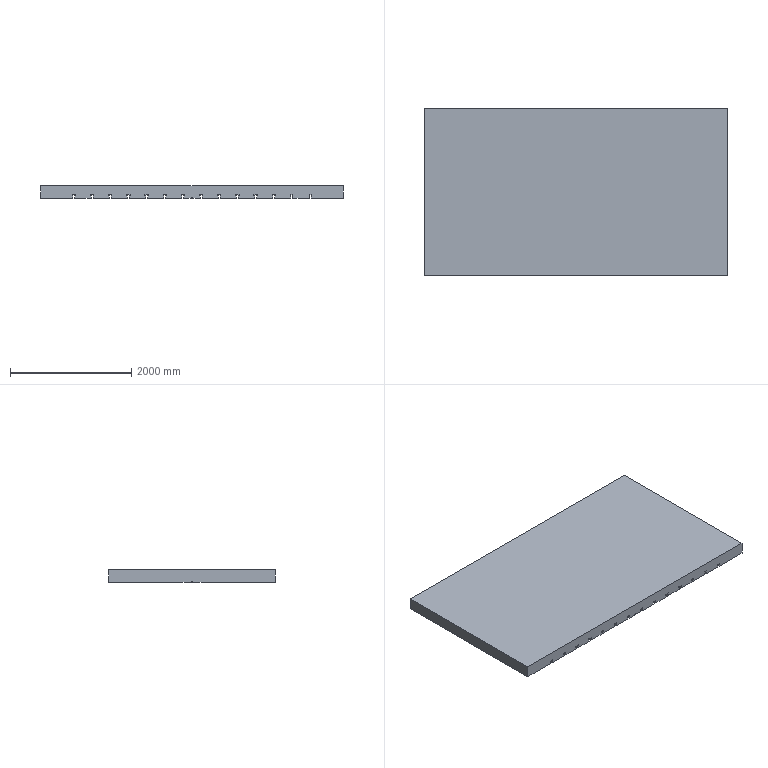Part | NX | features solid 2 | 1 solid | 178 faces | box 5000 x 2750 x 200 mm | volume 2661313760 mm3 | plane 178